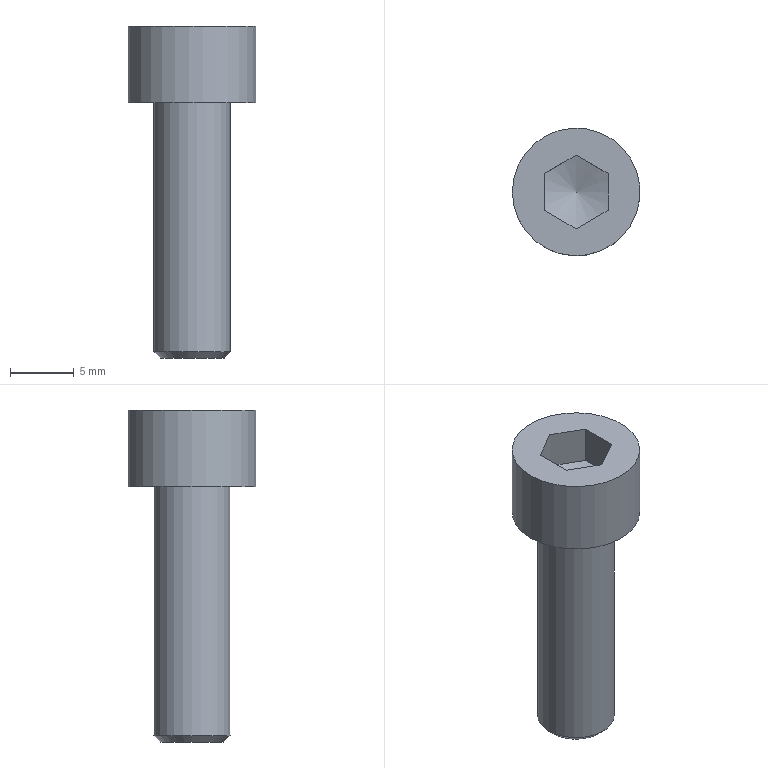Part | STEP file | 1_id130_xmt_txt | 1 solid | 19 faces | box 10 x 10 x 26 mm | volume 960.822 mm3 | plane 15 | cylinder 2 | cone 2 | commonest cylinder face diameters 6 x1 10 x1
STEP:
#1=CARTESIAN_POINT('',(110.,280.,101.));
#2=VERTEX_POINT('',#1);
#3=CARTESIAN_POINT('',(115.,280.,101.));
#4=DIRECTION('',(0.,0.,1.));
#5=DIRECTION('',(-1.,0.,0.));
#6=AXIS2_PLACEMENT_3D('',#3,#4,#5);
#7=CIRCLE('',#6,5.);
#8=EDGE_CURVE('',#2,#2,#7,.T.);
#9=ORIENTED_EDGE('',*,*,#8,.F.);
#10=EDGE_LOOP('',(#9));
#11=FACE_BOUND('',#10,.T.);
#12=CARTESIAN_POINT('',(110.,280.,95.));
#13=VERTEX_POINT('',#12);
#14=CARTESIAN_POINT('',(115.,280.,95.));
#15=DIRECTION('',(0.,0.,-1.));
#16=DIRECTION('',(-1.,0.,0.));
#17=AXIS2_PLACEMENT_3D('',#14,#15,#16);
#18=CIRCLE('',#17,5.);
#19=EDGE_CURVE('',#13,#13,#18,.T.);
#20=ORIENTED_EDGE('',*,*,#19,.F.);
#21=EDGE_LOOP('',(#20));
#22=FACE_BOUND('',#21,.T.);
#23=CARTESIAN_POINT('',(115.,280.,98.));
#24=DIRECTION('',(0.,0.,-1.));
#25=DIRECTION('',(1.,0.,0.));
#26=AXIS2_PLACEMENT_3D('',#23,#24,#25);
#27=CYLINDRICAL_SURFACE('',#26,5.);
#28=ADVANCED_FACE('',(#11,#22),#27,.T.);
#29=CARTESIAN_POINT('',(115.,282.887,98.));
#30=VERTEX_POINT('',#29);
#31=CARTESIAN_POINT('',(112.5,281.443,98.));
#32=VERTEX_POINT('',#31);
#33=CARTESIAN_POINT('',(115.,280.,98.));
#34=DIRECTION('',(0.,0.,1.));
#35=DIRECTION('',(-1.,0.,0.));
#36=AXIS2_PLACEMENT_3D('',#33,#34,#35);
#37=CIRCLE('',#36,2.887);
#38=EDGE_CURVE('',#30,#32,#37,.T.);
#39=ORIENTED_EDGE('',*,*,#38,.T.);
#40=CARTESIAN_POINT('',(112.5,278.557,98.));
#41=VERTEX_POINT('',#40);
#42=CARTESIAN_POINT('',(115.,280.,98.));
#43=DIRECTION('',(0.,0.,1.));
#44=DIRECTION('',(-1.,0.,0.));
#45=AXIS2_PLACEMENT_3D('',#42,#43,#44);
#46=CIRCLE('',#45,2.887);
#47=EDGE_CURVE('',#32,#41,#46,.T.);
#48=ORIENTED_EDGE('',*,*,#47,.T.);
#49=CARTESIAN_POINT('',(115.,277.113,98.));
#50=VERTEX_POINT('',#49);
#51=CARTESIAN_POINT('',(115.,280.,98.));
#52=DIRECTION('',(0.,0.,1.));
#53=DIRECTION('',(-1.,0.,0.));
#54=AXIS2_PLACEMENT_3D('',#51,#52,#53);
#55=CIRCLE('',#54,2.887);
#56=EDGE_CURVE('',#41,#50,#55,.T.);
#57=ORIENTED_EDGE('',*,*,#56,.T.);
#58=CARTESIAN_POINT('',(117.5,278.557,98.));
#59=VERTEX_POINT('',#58);
#60=CARTESIAN_POINT('',(115.,280.,98.));
#61=DIRECTION('',(0.,0.,1.));
#62=DIRECTION('',(-1.,0.,0.));
#63=AXIS2_PLACEMENT_3D('',#60,#61,#62);
#64=CIRCLE('',#63,2.887);
#65=EDGE_CURVE('',#50,#59,#64,.T.);
#66=ORIENTED_EDGE('',*,*,#65,.T.);
#67=CARTESIAN_POINT('',(117.5,281.443,98.));
#68=VERTEX_POINT('',#67);
#69=CARTESIAN_POINT('',(115.,280.,98.));
#70=DIRECTION('',(0.,0.,1.));
#71=DIRECTION('',(-1.,0.,0.));
#72=AXIS2_PLACEMENT_3D('',#69,#70,#71);
#73=CIRCLE('',#72,2.887);
#74=EDGE_CURVE('',#59,#68,#73,.T.);
#75=ORIENTED_EDGE('',*,*,#74,.T.);
#76=CARTESIAN_POINT('',(115.,280.,98.));
#77=DIRECTION('',(0.,0.,1.));
#78=DIRECTION('',(-1.,0.,0.));
#79=AXIS2_PLACEMENT_3D('',#76,#77,#78);
#80=CIRCLE('',#79,2.887);
#81=EDGE_CURVE('',#68,#30,#80,.T.);
#82=ORIENTED_EDGE('',*,*,#81,.T.);
#83=EDGE_LOOP('',(#39,#48,#57,#66,#75,#82));
#84=FACE_BOUND('',#83,.T.);
#85=CARTESIAN_POINT('',(115.,280.,97.));
#86=VERTEX_POINT('',#85);
#87=VERTEX_LOOP('',#86);
#88=FACE_BOUND('',#87,.T.);
#89=CARTESIAN_POINT('',(115.,280.,97.5));
#90=DIRECTION('',(0.,0.,1.));
#91=DIRECTION('',(1.,0.,0.));
#92=AXIS2_PLACEMENT_3D('',#89,#90,#91);
#93=CONICAL_SURFACE('',#92,1.443,70.893);
#94=ADVANCED_FACE('',(#84,#88),#93,.F.);
#95=CARTESIAN_POINT('',(112.,280.,95.));
#96=VERTEX_POINT('',#95);
#97=CARTESIAN_POINT('',(115.,280.,95.));
#98=DIRECTION('',(0.,0.,1.));
#99=DIRECTION('',(-1.,0.,0.));
#100=AXIS2_PLACEMENT_3D('',#97,#98,#99);
#101=CIRCLE('',#100,3.);
#102=EDGE_CURVE('',#96,#96,#101,.T.);
#103=ORIENTED_EDGE('',*,*,#102,.F.);
#104=EDGE_LOOP('',(#103));
#105=FACE_BOUND('',#104,.T.);
#106=CARTESIAN_POINT('',(118.,280.,75.5));
#107=VERTEX_POINT('',#106);
#108=CARTESIAN_POINT('',(115.,280.,75.5));
#109=DIRECTION('',(0.,0.,-1.));
#110=DIRECTION('',(1.,0.,0.));
#111=AXIS2_PLACEMENT_3D('',#108,#109,#110);
#112=CIRCLE('',#111,3.);
#113=EDGE_CURVE('',#107,#107,#112,.T.);
#114=ORIENTED_EDGE('',*,*,#113,.F.);
#115=EDGE_LOOP('',(#114));
#116=FACE_BOUND('',#115,.T.);
#117=CARTESIAN_POINT('',(115.,280.,85.));
#118=DIRECTION('',(0.,0.,-1.));
#119=DIRECTION('',(1.,0.,0.));
#120=AXIS2_PLACEMENT_3D('',#117,#118,#119);
#121=CYLINDRICAL_SURFACE('',#120,3.);
#122=ADVANCED_FACE('',(#105,#116),#121,.T.);
#123=ORIENTED_EDGE('',*,*,#113,.T.);
#124=EDGE_LOOP('',(#123));
#125=FACE_BOUND('',#124,.T.);
#126=CARTESIAN_POINT('',(117.5,280.,75.));
#127=VERTEX_POINT('',#126);
#128=CARTESIAN_POINT('',(115.,280.,75.));
#129=DIRECTION('',(0.,0.,1.));
#130=DIRECTION('',(1.,0.,0.));
#131=AXIS2_PLACEMENT_3D('',#128,#129,#130);
#132=CIRCLE('',#131,2.5);
#133=EDGE_CURVE('',#127,#127,#132,.T.);
#134=ORIENTED_EDGE('',*,*,#133,.T.);
#135=EDGE_LOOP('',(#134));
#136=FACE_BOUND('',#135,.T.);
#137=CARTESIAN_POINT('',(115.,280.,75.));
#138=DIRECTION('',(0.,0.,1.));
#139=DIRECTION('',(-1.,0.,0.));
#140=AXIS2_PLACEMENT_3D('',#137,#138,#139);
#141=CONICAL_SURFACE('',#140,2.5,45.);
#142=ADVANCED_FACE('',(#125,#136),#141,.T.);
#143=ORIENTED_EDGE('',*,*,#133,.F.);
#144=EDGE_LOOP('',(#143));
#145=FACE_OUTER_BOUND('',#144,.T.);
#146=CARTESIAN_POINT('',(115.,280.,75.));
#147=DIRECTION('',(0.,0.,-1.));
#148=DIRECTION('',(1.,0.,0.));
#149=AXIS2_PLACEMENT_3D('',#146,#147,#148);
#150=PLANE('',#149);
#151=ADVANCED_FACE('',(#145),#150,.T.);
#152=CARTESIAN_POINT('',(113.75,277.835,98.));
#153=DIRECTION('',(-0.866,0.5,0.));
#154=VECTOR('',#153,1.);
#155=LINE('',#152,#154);
#156=EDGE_CURVE('',#50,#41,#155,.T.);
#157=ORIENTED_EDGE('',*,*,#156,.F.);
#158=ORIENTED_EDGE('',*,*,#56,.F.);
#159=EDGE_LOOP('',(#157,#158));
#160=FACE_OUTER_BOUND('',#159,.T.);
#161=CARTESIAN_POINT('',(115.,280.,98.));
#162=DIRECTION('',(0.,0.,1.));
#163=DIRECTION('',(-1.,0.,0.));
#164=AXIS2_PLACEMENT_3D('',#161,#162,#163);
#165=PLANE('',#164);
#166=ADVANCED_FACE('',(#160),#165,.F.);
#167=CARTESIAN_POINT('',(112.5,280.,98.));
#168=DIRECTION('',(0.,1.,0.));
#169=VECTOR('',#168,1.);
#170=LINE('',#167,#169);
#171=EDGE_CURVE('',#41,#32,#170,.T.);
#172=ORIENTED_EDGE('',*,*,#171,.F.);
#173=ORIENTED_EDGE('',*,*,#47,.F.);
#174=EDGE_LOOP('',(#172,#173));
#175=FACE_OUTER_BOUND('',#174,.T.);
#176=CARTESIAN_POINT('',(115.,280.,98.));
#177=DIRECTION('',(0.,0.,1.));
#178=DIRECTION('',(-1.,0.,0.));
#179=AXIS2_PLACEMENT_3D('',#176,#177,#178);
#180=PLANE('',#179);
#181=ADVANCED_FACE('',(#175),#180,.F.);
#182=CARTESIAN_POINT('',(113.75,282.165,98.));
#183=DIRECTION('',(0.866,0.5,0.));
#184=VECTOR('',#183,1.);
#185=LINE('',#182,#184);
#186=EDGE_CURVE('',#32,#30,#185,.T.);
#187=ORIENTED_EDGE('',*,*,#186,.F.);
#188=ORIENTED_EDGE('',*,*,#38,.F.);
#189=EDGE_LOOP('',(#187,#188));
#190=FACE_OUTER_BOUND('',#189,.T.);
#191=CARTESIAN_POINT('',(115.,280.,98.));
#192=DIRECTION('',(0.,0.,1.));
#193=DIRECTION('',(-1.,0.,0.));
#194=AXIS2_PLACEMENT_3D('',#191,#192,#193);
#195=PLANE('',#194);
#196=ADVANCED_FACE('',(#190),#195,.F.);
#197=CARTESIAN_POINT('',(116.25,282.165,98.));
#198=DIRECTION('',(0.866,-0.5,0.));
#199=VECTOR('',#198,1.);
#200=LINE('',#197,#199);
#201=EDGE_CURVE('',#30,#68,#200,.T.);
#202=ORIENTED_EDGE('',*,*,#201,.F.);
#203=ORIENTED_EDGE('',*,*,#81,.F.);
#204=EDGE_LOOP('',(#202,#203));
#205=FACE_OUTER_BOUND('',#204,.T.);
#206=CARTESIAN_POINT('',(115.,280.,98.));
#207=DIRECTION('',(0.,0.,1.));
#208=DIRECTION('',(-1.,0.,0.));
#209=AXIS2_PLACEMENT_3D('',#206,#207,#208);
#210=PLANE('',#209);
#211=ADVANCED_FACE('',(#205),#210,.F.);
#212=CARTESIAN_POINT('',(117.5,280.,98.));
#213=DIRECTION('',(0.,-1.,0.));
#214=VECTOR('',#213,1.);
#215=LINE('',#212,#214);
#216=EDGE_CURVE('',#68,#59,#215,.T.);
#217=ORIENTED_EDGE('',*,*,#216,.F.);
#218=ORIENTED_EDGE('',*,*,#74,.F.);
#219=EDGE_LOOP('',(#217,#218));
#220=FACE_OUTER_BOUND('',#219,.T.);
#221=CARTESIAN_POINT('',(115.,280.,98.));
#222=DIRECTION('',(0.,0.,1.));
#223=DIRECTION('',(-1.,0.,0.));
#224=AXIS2_PLACEMENT_3D('',#221,#222,#223);
#225=PLANE('',#224);
#226=ADVANCED_FACE('',(#220),#225,.F.);
#227=CARTESIAN_POINT('',(116.25,277.835,98.));
#228=DIRECTION('',(-0.866,-0.5,0.));
#229=VECTOR('',#228,1.);
#230=LINE('',#227,#229);
#231=EDGE_CURVE('',#59,#50,#230,.T.);
#232=ORIENTED_EDGE('',*,*,#231,.F.);
#233=ORIENTED_EDGE('',*,*,#65,.F.);
#234=EDGE_LOOP('',(#232,#233));
#235=FACE_OUTER_BOUND('',#234,.T.);
#236=CARTESIAN_POINT('',(115.,280.,98.));
#237=DIRECTION('',(0.,0.,1.));
#238=DIRECTION('',(-1.,0.,0.));
#239=AXIS2_PLACEMENT_3D('',#236,#237,#238);
#240=PLANE('',#239);
#241=ADVANCED_FACE('',(#235),#240,.F.);
#242=CARTESIAN_POINT('',(115.,277.113,101.));
#243=VERTEX_POINT('',#242);
#244=CARTESIAN_POINT('',(115.,277.113,99.5));
#245=DIRECTION('',(0.,0.,1.));
#246=VECTOR('',#245,1.);
#247=LINE('',#244,#246);
#248=EDGE_CURVE('',#50,#243,#247,.T.);
#249=ORIENTED_EDGE('',*,*,#248,.F.);
#250=ORIENTED_EDGE('',*,*,#156,.T.);
#251=CARTESIAN_POINT('',(112.5,278.557,101.));
#252=VERTEX_POINT('',#251);
#253=CARTESIAN_POINT('',(112.5,278.557,99.5));
#254=DIRECTION('',(0.,0.,1.));
#255=VECTOR('',#254,1.);
#256=LINE('',#253,#255);
#257=EDGE_CURVE('',#41,#252,#256,.T.);
#258=ORIENTED_EDGE('',*,*,#257,.T.);
#259=CARTESIAN_POINT('',(113.75,277.835,101.));
#260=DIRECTION('',(-0.866,0.5,0.));
#261=VECTOR('',#260,1.);
#262=LINE('',#259,#261);
#263=EDGE_CURVE('',#243,#252,#262,.T.);
#264=ORIENTED_EDGE('',*,*,#263,.F.);
#265=EDGE_LOOP('',(#249,#250,#258,#264));
#266=FACE_OUTER_BOUND('',#265,.T.);
#267=CARTESIAN_POINT('',(113.75,277.835,99.5));
#268=DIRECTION('',(0.5,0.866,0.));
#269=DIRECTION('',(0.,0.,1.));
#270=AXIS2_PLACEMENT_3D('',#267,#268,#269);
#271=PLANE('',#270);
#272=ADVANCED_FACE('',(#266),#271,.T.);
#273=CARTESIAN_POINT('',(117.5,278.557,101.));
#274=VERTEX_POINT('',#273);
#275=CARTESIAN_POINT('',(117.5,278.557,99.5));
#276=DIRECTION('',(0.,0.,1.));
#277=VECTOR('',#276,1.);
#278=LINE('',#275,#277);
#279=EDGE_CURVE('',#59,#274,#278,.T.);
#280=ORIENTED_EDGE('',*,*,#279,.F.);
#281=ORIENTED_EDGE('',*,*,#231,.T.);
#282=ORIENTED_EDGE('',*,*,#248,.T.);
#283=CARTESIAN_POINT('',(116.25,277.835,101.));
#284=DIRECTION('',(-0.866,-0.5,0.));
#285=VECTOR('',#284,1.);
#286=LINE('',#283,#285);
#287=EDGE_CURVE('',#274,#243,#286,.T.);
#288=ORIENTED_EDGE('',*,*,#287,.F.);
#289=EDGE_LOOP('',(#280,#281,#282,#288));
#290=FACE_OUTER_BOUND('',#289,.T.);
#291=CARTESIAN_POINT('',(116.25,277.835,99.5));
#292=DIRECTION('',(-0.5,0.866,0.));
#293=DIRECTION('',(0.,0.,-1.));
#294=AXIS2_PLACEMENT_3D('',#291,#292,#293);
#295=PLANE('',#294);
#296=ADVANCED_FACE('',(#290),#295,.T.);
#297=CARTESIAN_POINT('',(117.5,281.443,101.));
#298=VERTEX_POINT('',#297);
#299=CARTESIAN_POINT('',(117.5,281.443,99.5));
#300=DIRECTION('',(0.,0.,1.));
#301=VECTOR('',#300,1.);
#302=LINE('',#299,#301);
#303=EDGE_CURVE('',#68,#298,#302,.T.);
#304=ORIENTED_EDGE('',*,*,#303,.F.);
#305=ORIENTED_EDGE('',*,*,#216,.T.);
#306=ORIENTED_EDGE('',*,*,#279,.T.);
#307=CARTESIAN_POINT('',(117.5,280.,101.));
#308=DIRECTION('',(0.,-1.,0.));
#309=VECTOR('',#308,1.);
#310=LINE('',#307,#309);
#311=EDGE_CURVE('',#298,#274,#310,.T.);
#312=ORIENTED_EDGE('',*,*,#311,.F.);
#313=EDGE_LOOP('',(#304,#305,#306,#312));
#314=FACE_OUTER_BOUND('',#313,.T.);
#315=CARTESIAN_POINT('',(117.5,280.,99.5));
#316=DIRECTION('',(-1.,0.,0.));
#317=DIRECTION('',(0.,0.,-1.));
#318=AXIS2_PLACEMENT_3D('',#315,#316,#317);
#319=PLANE('',#318);
#320=ADVANCED_FACE('',(#314),#319,.T.);
#321=CARTESIAN_POINT('',(115.,282.887,101.));
#322=VERTEX_POINT('',#321);
#323=CARTESIAN_POINT('',(115.,282.887,99.5));
#324=DIRECTION('',(0.,0.,1.));
#325=VECTOR('',#324,1.);
#326=LINE('',#323,#325);
#327=EDGE_CURVE('',#30,#322,#326,.T.);
#328=ORIENTED_EDGE('',*,*,#327,.F.);
#329=ORIENTED_EDGE('',*,*,#201,.T.);
#330=ORIENTED_EDGE('',*,*,#303,.T.);
#331=CARTESIAN_POINT('',(116.25,282.165,101.));
#332=DIRECTION('',(0.866,-0.5,0.));
#333=VECTOR('',#332,1.);
#334=LINE('',#331,#333);
#335=EDGE_CURVE('',#322,#298,#334,.T.);
#336=ORIENTED_EDGE('',*,*,#335,.F.);
#337=EDGE_LOOP('',(#328,#329,#330,#336));
#338=FACE_OUTER_BOUND('',#337,.T.);
#339=CARTESIAN_POINT('',(116.25,282.165,99.5));
#340=DIRECTION('',(-0.5,-0.866,0.));
#341=DIRECTION('',(0.,0.,-1.));
#342=AXIS2_PLACEMENT_3D('',#339,#340,#341);
#343=PLANE('',#342);
#344=ADVANCED_FACE('',(#338),#343,.T.);
#345=CARTESIAN_POINT('',(112.5,281.443,101.));
#346=VERTEX_POINT('',#345);
#347=CARTESIAN_POINT('',(112.5,281.443,99.5));
#348=DIRECTION('',(0.,0.,1.));
#349=VECTOR('',#348,1.);
#350=LINE('',#347,#349);
#351=EDGE_CURVE('',#32,#346,#350,.T.);
#352=ORIENTED_EDGE('',*,*,#351,.F.);
#353=ORIENTED_EDGE('',*,*,#186,.T.);
#354=ORIENTED_EDGE('',*,*,#327,.T.);
#355=CARTESIAN_POINT('',(113.75,282.165,101.));
#356=DIRECTION('',(0.866,0.5,0.));
#357=VECTOR('',#356,1.);
#358=LINE('',#355,#357);
#359=EDGE_CURVE('',#346,#322,#358,.T.);
#360=ORIENTED_EDGE('',*,*,#359,.F.);
#361=EDGE_LOOP('',(#352,#353,#354,#360));
#362=FACE_OUTER_BOUND('',#361,.T.);
#363=CARTESIAN_POINT('',(113.75,282.165,99.5));
#364=DIRECTION('',(0.5,-0.866,0.));
#365=DIRECTION('',(0.,0.,1.));
#366=AXIS2_PLACEMENT_3D('',#363,#364,#365);
#367=PLANE('',#366);
#368=ADVANCED_FACE('',(#362),#367,.T.);
#369=ORIENTED_EDGE('',*,*,#257,.F.);
#370=ORIENTED_EDGE('',*,*,#171,.T.);
#371=ORIENTED_EDGE('',*,*,#351,.T.);
#372=CARTESIAN_POINT('',(112.5,280.,101.));
#373=DIRECTION('',(0.,1.,0.));
#374=VECTOR('',#373,1.);
#375=LINE('',#372,#374);
#376=EDGE_CURVE('',#252,#346,#375,.T.);
#377=ORIENTED_EDGE('',*,*,#376,.F.);
#378=EDGE_LOOP('',(#369,#370,#371,#377));
#379=FACE_OUTER_BOUND('',#378,.T.);
#380=CARTESIAN_POINT('',(112.5,280.,99.5));
#381=DIRECTION('',(1.,0.,0.));
#382=DIRECTION('',(0.,0.,1.));
#383=AXIS2_PLACEMENT_3D('',#380,#381,#382);
#384=PLANE('',#383);
#385=ADVANCED_FACE('',(#379),#384,.T.);
#386=ORIENTED_EDGE('',*,*,#263,.T.);
#387=ORIENTED_EDGE('',*,*,#376,.T.);
#388=ORIENTED_EDGE('',*,*,#359,.T.);
#389=ORIENTED_EDGE('',*,*,#335,.T.);
#390=ORIENTED_EDGE('',*,*,#311,.T.);
#391=ORIENTED_EDGE('',*,*,#287,.T.);
#392=EDGE_LOOP('',(#386,#387,#388,#389,#390,#391));
#393=FACE_BOUND('',#392,.T.);
#394=ORIENTED_EDGE('',*,*,#8,.T.);
#395=EDGE_LOOP('',(#394));
#396=FACE_BOUND('',#395,.T.);
#397=CARTESIAN_POINT('',(115.,280.,101.));
#398=DIRECTION('',(0.,0.,1.));
#399=DIRECTION('',(-1.,0.,0.));
#400=AXIS2_PLACEMENT_3D('',#397,#398,#399);
#401=PLANE('',#400);
#402=ADVANCED_FACE('',(#393,#396),#401,.T.);
#403=ORIENTED_EDGE('',*,*,#102,.T.);
#404=EDGE_LOOP('',(#403));
#405=FACE_BOUND('',#404,.T.);
#406=ORIENTED_EDGE('',*,*,#19,.T.);
#407=EDGE_LOOP('',(#406));
#408=FACE_BOUND('',#407,.T.);
#409=CARTESIAN_POINT('',(115.,280.,95.));
#410=DIRECTION('',(0.,0.,-1.));
#411=DIRECTION('',(1.,0.,0.));
#412=AXIS2_PLACEMENT_3D('',#409,#410,#411);
#413=PLANE('',#412);
#414=ADVANCED_FACE('',(#405,#408),#413,.T.);
#415=CLOSED_SHELL('',(#28,#94,#122,#142,#151,#166,#181,#196,#211,#226,#241,#272,#296,#320,#344,#368,#385,#402,#414));
#416=MANIFOLD_SOLID_BREP('',#415);
#417=(LENGTH_UNIT()NAMED_UNIT(*)SI_UNIT(.MILLI.,.METRE.));
#418=UNCERTAINTY_MEASURE_WITH_UNIT(LENGTH_MEASURE(0.00002),#417,'','');
#419=(NAMED_UNIT(*)PLANE_ANGLE_UNIT()SI_UNIT($,.RADIAN.));
#420=PLANE_ANGLE_MEASURE_WITH_UNIT(PLANE_ANGLE_MEASURE(0.01745),#419);
#421=DIMENSIONAL_EXPONENTS(0.,0.,0.,0.,0.,0.,0.);
#422=(CONVERSION_BASED_UNIT('DEGREE',#420)NAMED_UNIT(#421)PLANE_ANGLE_UNIT());
#423=(NAMED_UNIT(*)SI_UNIT($,.STERADIAN.)SOLID_ANGLE_UNIT());
#424=(GEOMETRIC_REPRESENTATION_CONTEXT(3)GLOBAL_UNCERTAINTY_ASSIGNED_CONTEXT((#418))GLOBAL_UNIT_ASSIGNED_CONTEXT((#417,#422,#423))REPRESENTATION_CONTEXT('',''));
#425=ADVANCED_BREP_SHAPE_REPRESENTATION('',(#416),#424);